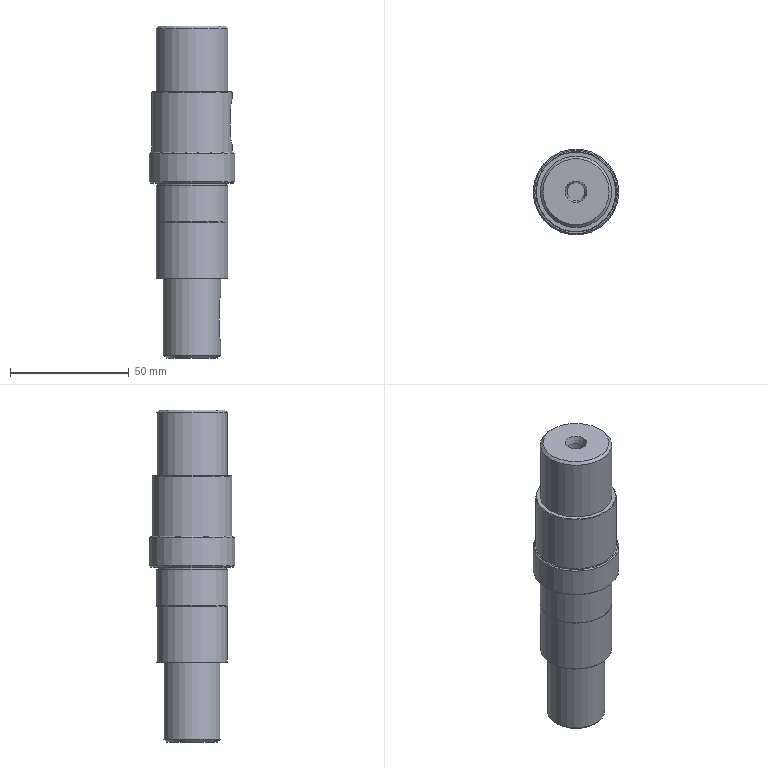Part | NX | features CHAMFER 9, CYLINDER 6, DATUM_CSYS 3, DATUM_PLANE 2, EXTRUDE 2, SKETCH 2, U_SLOT 2, RECT_GROOVE 1, Resize Face 1 | 6 solids | 51 faces | box 36 x 36 x 139.56 mm | volume 97541 mm3 | plane 21 | cylinder 17 | cone 9 | torus 4 | commonest cylinder face diameters 0.8 x2 1 x2 8 x2 10 x2 30 x2 7.48 x1
STEP:
#1=CARTESIAN_POINT('',(-12.04,0.,-110.72));
#2=VERTEX_POINT('',#1);
#3=CARTESIAN_POINT('',(0.,0.,-110.72));
#4=DIRECTION('',(0.,0.,-1.));
#5=DIRECTION('',(-1.,0.,0.));
#6=AXIS2_PLACEMENT_3D('',#3,#4,#5);
#7=CIRCLE('',#6,12.04);
#8=EDGE_CURVE('',#2,#2,#7,.F.);
#9=ORIENTED_EDGE('',*,*,#8,.T.);
#10=EDGE_LOOP('',(#9));
#11=FACE_BOUND('',#10,.T.);
#12=CARTESIAN_POINT('',(11.356,-4.,-89.51));
#13=VERTEX_POINT('',#12);
#14=CARTESIAN_POINT('',(11.356,-4.,-101.11));
#15=VERTEX_POINT('',#14);
#16=CARTESIAN_POINT('',(11.356,-4.,-78.7));
#17=DIRECTION('',(0.,0.,-1.));
#18=VECTOR('',#17,1000.);
#19=LINE('',#16,#18);
#20=EDGE_CURVE('',#13,#15,#19,.T.);
#21=ORIENTED_EDGE('',*,*,#20,.F.);
#22=CARTESIAN_POINT('',(11.356,4.,-89.51));
#23=VERTEX_POINT('',#22);
#24=CARTESIAN_POINT('',(11.356,4.,-89.51));
#25=CARTESIAN_POINT('',(11.356,4.,-88.445));
#26=CARTESIAN_POINT('',(11.708,3.133,-86.386));
#27=CARTESIAN_POINT('',(12.206,0.006902,-85.072));
#28=CARTESIAN_POINT('',(11.708,-3.135,-86.384));
#29=CARTESIAN_POINT('',(11.356,-4.,-88.445));
#30=CARTESIAN_POINT('',(11.356,-4.,-89.51));
#31=B_SPLINE_CURVE_WITH_KNOTS('',3,(#24,#25,#26,#27,#28,#29,#30),.UNSPECIFIED.,.F.,.F.,(4,1,1,1,4),(0.,0.003148,0.006295,0.009443,0.01259),.UNSPECIFIED.);
#32=EDGE_CURVE('',#23,#13,#31,.T.);
#33=ORIENTED_EDGE('',*,*,#32,.F.);
#34=CARTESIAN_POINT('',(11.356,4.,-101.11));
#35=VERTEX_POINT('',#34);
#36=CARTESIAN_POINT('',(11.356,4.,-78.7));
#37=DIRECTION('',(0.,0.,-1.));
#38=VECTOR('',#37,1000.);
#39=LINE('',#36,#38);
#40=EDGE_CURVE('',#35,#23,#39,.F.);
#41=ORIENTED_EDGE('',*,*,#40,.F.);
#42=CARTESIAN_POINT('',(11.356,-4.,-101.11));
#43=CARTESIAN_POINT('',(11.356,-4.,-102.175));
#44=CARTESIAN_POINT('',(11.708,-3.133,-104.234));
#45=CARTESIAN_POINT('',(12.206,-0.006902,-105.548));
#46=CARTESIAN_POINT('',(11.708,3.135,-104.236));
#47=CARTESIAN_POINT('',(11.356,4.,-102.175));
#48=CARTESIAN_POINT('',(11.356,4.,-101.11));
#49=B_SPLINE_CURVE_WITH_KNOTS('',3,(#42,#43,#44,#45,#46,#47,#48),.UNSPECIFIED.,.F.,.F.,(4,1,1,1,4),(0.,0.003148,0.006295,0.009443,0.01259),.UNSPECIFIED.);
#50=EDGE_CURVE('',#15,#35,#49,.T.);
#51=ORIENTED_EDGE('',*,*,#50,.F.);
#52=EDGE_LOOP('',(#21,#33,#41,#51));
#53=FACE_BOUND('',#52,.T.);
#54=CARTESIAN_POINT('',(12.04,0.,-78.7));
#55=VERTEX_POINT('',#54);
#56=CARTESIAN_POINT('',(0.,0.,-78.7));
#57=DIRECTION('',(0.,0.,-1.));
#58=DIRECTION('',(1.,0.,0.));
#59=AXIS2_PLACEMENT_3D('',#56,#57,#58);
#60=CIRCLE('',#59,12.04);
#61=EDGE_CURVE('',#55,#55,#60,.T.);
#62=ORIENTED_EDGE('',*,*,#61,.T.);
#63=EDGE_LOOP('',(#62));
#64=FACE_BOUND('',#63,.T.);
#65=CARTESIAN_POINT('',(0.,0.,-78.7));
#66=DIRECTION('',(0.,0.,-1.));
#67=DIRECTION('',(1.,0.,0.));
#68=AXIS2_PLACEMENT_3D('',#65,#66,#67);
#69=CYLINDRICAL_SURFACE('',#68,12.04);
#70=ADVANCED_FACE('',(#11,#53,#64),#69,.T.);
#71=CARTESIAN_POINT('',(-10.84,0.,-111.92));
#72=VERTEX_POINT('',#71);
#73=CARTESIAN_POINT('',(0.,0.,-111.92));
#74=DIRECTION('',(0.,0.,-1.));
#75=DIRECTION('',(-1.,0.,0.));
#76=AXIS2_PLACEMENT_3D('',#73,#74,#75);
#77=CIRCLE('',#76,10.84);
#78=EDGE_CURVE('',#72,#72,#77,.T.);
#79=ORIENTED_EDGE('',*,*,#78,.T.);
#80=EDGE_LOOP('',(#79));
#81=FACE_BOUND('',#80,.T.);
#82=CARTESIAN_POINT('',(-4.84,0.,-111.92));
#83=VERTEX_POINT('',#82);
#84=CARTESIAN_POINT('',(0.,0.,-111.92));
#85=DIRECTION('',(0.,0.,-1.));
#86=DIRECTION('',(-1.,0.,0.));
#87=AXIS2_PLACEMENT_3D('',#84,#85,#86);
#88=CIRCLE('',#87,4.84);
#89=EDGE_CURVE('',#83,#83,#88,.F.);
#90=ORIENTED_EDGE('',*,*,#89,.T.);
#91=EDGE_LOOP('',(#90));
#92=FACE_BOUND('',#91,.T.);
#93=CARTESIAN_POINT('',(0.,0.,-111.92));
#94=DIRECTION('',(0.,0.,-1.));
#95=DIRECTION('',(-1.,0.,0.));
#96=AXIS2_PLACEMENT_3D('',#93,#94,#95);
#97=PLANE('',#96);
#98=ADVANCED_FACE('',(#81,#92),#97,.T.);
#99=ORIENTED_EDGE('',*,*,#61,.F.);
#100=EDGE_LOOP('',(#99));
#101=FACE_BOUND('',#100,.T.);
#102=CARTESIAN_POINT('',(0.,0.,-78.7));
#103=DIRECTION('',(0.,0.,1.));
#104=DIRECTION('',(1.,0.,0.));
#105=AXIS2_PLACEMENT_3D('',#102,#103,#104);
#106=PLANE('',#105);
#107=ADVANCED_FACE('',(#101),#106,.T.);
#108=CARTESIAN_POINT('',(-4.04,0.,-108.72));
#109=VERTEX_POINT('',#108);
#110=CARTESIAN_POINT('',(0.,0.,-108.72));
#111=DIRECTION('',(0.,0.,-1.));
#112=DIRECTION('',(-1.,0.,0.));
#113=AXIS2_PLACEMENT_3D('',#110,#111,#112);
#114=CIRCLE('',#113,4.04);
#115=EDGE_CURVE('',#109,#109,#114,.T.);
#116=ORIENTED_EDGE('',*,*,#115,.T.);
#117=EDGE_LOOP('',(#116));
#118=FACE_BOUND('',#117,.T.);
#119=CARTESIAN_POINT('',(4.04,0.,-107.02));
#120=VERTEX_POINT('',#119);
#121=CARTESIAN_POINT('',(0.,0.,-107.02));
#122=DIRECTION('',(0.,0.,-1.));
#123=DIRECTION('',(1.,0.,0.));
#124=AXIS2_PLACEMENT_3D('',#121,#122,#123);
#125=CIRCLE('',#124,4.04);
#126=EDGE_CURVE('',#120,#120,#125,.F.);
#127=ORIENTED_EDGE('',*,*,#126,.T.);
#128=EDGE_LOOP('',(#127));
#129=FACE_BOUND('',#128,.T.);
#130=CARTESIAN_POINT('',(0.,0.,-107.02));
#131=DIRECTION('',(0.,0.,-1.));
#132=DIRECTION('',(-1.,0.,0.));
#133=AXIS2_PLACEMENT_3D('',#130,#131,#132);
#134=CYLINDRICAL_SURFACE('',#133,4.04);
#135=ADVANCED_FACE('',(#118,#129),#134,.F.);
#136=ORIENTED_EDGE('',*,*,#126,.F.);
#137=EDGE_LOOP('',(#136));
#138=FACE_BOUND('',#137,.T.);
#139=CARTESIAN_POINT('',(0.,0.,-107.02));
#140=DIRECTION('',(0.,0.,-1.));
#141=DIRECTION('',(-1.,0.,0.));
#142=AXIS2_PLACEMENT_3D('',#139,#140,#141);
#143=PLANE('',#142);
#144=ADVANCED_FACE('',(#138),#143,.T.);
#145=ORIENTED_EDGE('',*,*,#89,.F.);
#146=EDGE_LOOP('',(#145));
#147=FACE_BOUND('',#146,.T.);
#148=ORIENTED_EDGE('',*,*,#115,.F.);
#149=EDGE_LOOP('',(#148));
#150=FACE_BOUND('',#149,.T.);
#151=CARTESIAN_POINT('',(0.,0.,-108.72));
#152=DIRECTION('',(0.,0.,-1.));
#153=DIRECTION('',(-1.,0.,0.));
#154=AXIS2_PLACEMENT_3D('',#151,#152,#153);
#155=CONICAL_SURFACE('',#154,4.04,0.245);
#156=ADVANCED_FACE('',(#147,#150),#155,.F.);
#157=ORIENTED_EDGE('',*,*,#20,.T.);
#158=CARTESIAN_POINT('',(9.34,-4.,-101.11));
#159=VERTEX_POINT('',#158);
#160=CARTESIAN_POINT('',(12.04,-4.,-101.11));
#161=DIRECTION('',(1.,0.,0.));
#162=VECTOR('',#161,1000.);
#163=LINE('',#160,#162);
#164=EDGE_CURVE('',#15,#159,#163,.F.);
#165=ORIENTED_EDGE('',*,*,#164,.T.);
#166=CARTESIAN_POINT('',(9.34,-4.,-89.51));
#167=VERTEX_POINT('',#166);
#168=CARTESIAN_POINT('',(9.34,-4.,-101.11));
#169=DIRECTION('',(0.,0.,1.));
#170=VECTOR('',#169,1000.);
#171=LINE('',#168,#170);
#172=EDGE_CURVE('',#167,#159,#171,.F.);
#173=ORIENTED_EDGE('',*,*,#172,.F.);
#174=CARTESIAN_POINT('',(12.04,-4.,-89.51));
#175=DIRECTION('',(1.,0.,0.));
#176=VECTOR('',#175,1000.);
#177=LINE('',#174,#176);
#178=EDGE_CURVE('',#13,#167,#177,.F.);
#179=ORIENTED_EDGE('',*,*,#178,.F.);
#180=EDGE_LOOP('',(#157,#165,#173,#179));
#181=FACE_BOUND('',#180,.T.);
#182=CARTESIAN_POINT('',(12.04,-4.,-95.31));
#183=DIRECTION('',(0.,-1.,0.));
#184=DIRECTION('',(0.,0.,-1.));
#185=AXIS2_PLACEMENT_3D('',#182,#183,#184);
#186=PLANE('',#185);
#187=ADVANCED_FACE('',(#181),#186,.F.);
#188=ORIENTED_EDGE('',*,*,#172,.T.);
#189=CARTESIAN_POINT('',(8.94,-3.6,-101.11));
#190=VERTEX_POINT('',#189);
#191=CARTESIAN_POINT('',(9.34,-3.6,-101.11));
#192=DIRECTION('',(0.,0.,1.));
#193=DIRECTION('',(1.,0.,0.));
#194=AXIS2_PLACEMENT_3D('',#191,#192,#193);
#195=CIRCLE('',#194,0.4);
#196=EDGE_CURVE('',#159,#190,#195,.F.);
#197=ORIENTED_EDGE('',*,*,#196,.T.);
#198=CARTESIAN_POINT('',(8.94,-3.6,-89.51));
#199=VERTEX_POINT('',#198);
#200=CARTESIAN_POINT('',(8.94,-3.6,-95.31));
#201=DIRECTION('',(0.,0.,1.));
#202=VECTOR('',#201,1000.);
#203=LINE('',#200,#202);
#204=EDGE_CURVE('',#199,#190,#203,.F.);
#205=ORIENTED_EDGE('',*,*,#204,.F.);
#206=CARTESIAN_POINT('',(9.34,-3.6,-89.51));
#207=DIRECTION('',(0.,0.,1.));
#208=DIRECTION('',(1.,0.,0.));
#209=AXIS2_PLACEMENT_3D('',#206,#207,#208);
#210=CIRCLE('',#209,0.4);
#211=EDGE_CURVE('',#167,#199,#210,.F.);
#212=ORIENTED_EDGE('',*,*,#211,.F.);
#213=EDGE_LOOP('',(#188,#197,#205,#212));
#214=FACE_BOUND('',#213,.T.);
#215=CARTESIAN_POINT('',(9.34,-3.6,-95.31));
#216=DIRECTION('',(0.,0.,1.));
#217=DIRECTION('',(1.,0.,0.));
#218=AXIS2_PLACEMENT_3D('',#215,#216,#217);
#219=CYLINDRICAL_SURFACE('',#218,0.4);
#220=ADVANCED_FACE('',(#214),#219,.F.);
#221=ORIENTED_EDGE('',*,*,#204,.T.);
#222=CARTESIAN_POINT('',(8.94,3.6,-101.11));
#223=VERTEX_POINT('',#222);
#224=CARTESIAN_POINT('',(8.94,0.,-101.11));
#225=DIRECTION('',(1.,0.,0.));
#226=DIRECTION('',(0.,0.,-1.));
#227=AXIS2_PLACEMENT_3D('',#224,#225,#226);
#228=CIRCLE('',#227,3.6);
#229=EDGE_CURVE('',#223,#190,#228,.F.);
#230=ORIENTED_EDGE('',*,*,#229,.F.);
#231=CARTESIAN_POINT('',(8.94,3.6,-89.51));
#232=VERTEX_POINT('',#231);
#233=CARTESIAN_POINT('',(8.94,3.6,-95.31));
#234=DIRECTION('',(0.,0.,1.));
#235=VECTOR('',#234,1000.);
#236=LINE('',#233,#235);
#237=EDGE_CURVE('',#232,#223,#236,.F.);
#238=ORIENTED_EDGE('',*,*,#237,.F.);
#239=CARTESIAN_POINT('',(8.94,0.,-89.51));
#240=DIRECTION('',(1.,0.,0.));
#241=DIRECTION('',(0.,0.,-1.));
#242=AXIS2_PLACEMENT_3D('',#239,#240,#241);
#243=CIRCLE('',#242,3.6);
#244=EDGE_CURVE('',#199,#232,#243,.F.);
#245=ORIENTED_EDGE('',*,*,#244,.F.);
#246=EDGE_LOOP('',(#221,#230,#238,#245));
#247=FACE_BOUND('',#246,.T.);
#248=CARTESIAN_POINT('',(8.94,0.,-95.31));
#249=DIRECTION('',(-1.,0.,0.));
#250=DIRECTION('',(0.,0.,1.));
#251=AXIS2_PLACEMENT_3D('',#248,#249,#250);
#252=PLANE('',#251);
#253=ADVANCED_FACE('',(#247),#252,.F.);
#254=ORIENTED_EDGE('',*,*,#237,.T.);
#255=CARTESIAN_POINT('',(9.34,4.,-101.11));
#256=VERTEX_POINT('',#255);
#257=CARTESIAN_POINT('',(9.34,3.6,-101.11));
#258=DIRECTION('',(0.,0.,1.));
#259=DIRECTION('',(1.,0.,0.));
#260=AXIS2_PLACEMENT_3D('',#257,#258,#259);
#261=CIRCLE('',#260,0.4);
#262=EDGE_CURVE('',#223,#256,#261,.F.);
#263=ORIENTED_EDGE('',*,*,#262,.T.);
#264=CARTESIAN_POINT('',(9.34,4.,-89.51));
#265=VERTEX_POINT('',#264);
#266=CARTESIAN_POINT('',(9.34,4.,-101.11));
#267=DIRECTION('',(0.,0.,1.));
#268=VECTOR('',#267,1000.);
#269=LINE('',#266,#268);
#270=EDGE_CURVE('',#265,#256,#269,.F.);
#271=ORIENTED_EDGE('',*,*,#270,.F.);
#272=CARTESIAN_POINT('',(9.34,3.6,-89.51));
#273=DIRECTION('',(0.,0.,1.));
#274=DIRECTION('',(1.,0.,0.));
#275=AXIS2_PLACEMENT_3D('',#272,#273,#274);
#276=CIRCLE('',#275,0.4);
#277=EDGE_CURVE('',#232,#265,#276,.F.);
#278=ORIENTED_EDGE('',*,*,#277,.F.);
#279=EDGE_LOOP('',(#254,#263,#271,#278));
#280=FACE_BOUND('',#279,.T.);
#281=CARTESIAN_POINT('',(9.34,3.6,-95.31));
#282=DIRECTION('',(0.,0.,1.));
#283=DIRECTION('',(1.,0.,0.));
#284=AXIS2_PLACEMENT_3D('',#281,#282,#283);
#285=CYLINDRICAL_SURFACE('',#284,0.4);
#286=ADVANCED_FACE('',(#280),#285,.F.);
#287=ORIENTED_EDGE('',*,*,#32,.T.);
#288=ORIENTED_EDGE('',*,*,#178,.T.);
#289=CARTESIAN_POINT('',(9.34,0.,-89.51));
#290=DIRECTION('',(1.,0.,0.));
#291=DIRECTION('',(0.,0.,-1.));
#292=AXIS2_PLACEMENT_3D('',#289,#290,#291);
#293=CIRCLE('',#292,4.);
#294=EDGE_CURVE('',#167,#265,#293,.F.);
#295=ORIENTED_EDGE('',*,*,#294,.T.);
#296=CARTESIAN_POINT('',(12.04,4.,-89.51));
#297=DIRECTION('',(1.,0.,0.));
#298=VECTOR('',#297,1000.);
#299=LINE('',#296,#298);
#300=EDGE_CURVE('',#23,#265,#299,.F.);
#301=ORIENTED_EDGE('',*,*,#300,.F.);
#302=EDGE_LOOP('',(#287,#288,#295,#301));
#303=FACE_BOUND('',#302,.T.);
#304=CARTESIAN_POINT('',(12.04,0.,-89.51));
#305=DIRECTION('',(1.,0.,0.));
#306=DIRECTION('',(0.,0.,-1.));
#307=AXIS2_PLACEMENT_3D('',#304,#305,#306);
#308=CYLINDRICAL_SURFACE('',#307,4.);
#309=ADVANCED_FACE('',(#303),#308,.F.);
#310=ORIENTED_EDGE('',*,*,#40,.T.);
#311=ORIENTED_EDGE('',*,*,#300,.T.);
#312=ORIENTED_EDGE('',*,*,#270,.T.);
#313=CARTESIAN_POINT('',(12.04,4.,-101.11));
#314=DIRECTION('',(1.,0.,0.));
#315=VECTOR('',#314,1000.);
#316=LINE('',#313,#315);
#317=EDGE_CURVE('',#35,#256,#316,.F.);
#318=ORIENTED_EDGE('',*,*,#317,.F.);
#319=EDGE_LOOP('',(#310,#311,#312,#318));
#320=FACE_BOUND('',#319,.T.);
#321=CARTESIAN_POINT('',(12.04,4.,-95.31));
#322=DIRECTION('',(0.,1.,0.));
#323=DIRECTION('',(0.,0.,1.));
#324=AXIS2_PLACEMENT_3D('',#321,#322,#323);
#325=PLANE('',#324);
#326=ADVANCED_FACE('',(#320),#325,.F.);
#327=ORIENTED_EDGE('',*,*,#164,.F.);
#328=ORIENTED_EDGE('',*,*,#50,.T.);
#329=ORIENTED_EDGE('',*,*,#317,.T.);
#330=CARTESIAN_POINT('',(9.34,0.,-101.11));
#331=DIRECTION('',(1.,0.,0.));
#332=DIRECTION('',(0.,0.,-1.));
#333=AXIS2_PLACEMENT_3D('',#330,#331,#332);
#334=CIRCLE('',#333,4.);
#335=EDGE_CURVE('',#256,#159,#334,.F.);
#336=ORIENTED_EDGE('',*,*,#335,.T.);
#337=EDGE_LOOP('',(#327,#328,#329,#336));
#338=FACE_BOUND('',#337,.T.);
#339=CARTESIAN_POINT('',(12.04,0.,-101.11));
#340=DIRECTION('',(1.,0.,0.));
#341=DIRECTION('',(0.,0.,-1.));
#342=AXIS2_PLACEMENT_3D('',#339,#340,#341);
#343=CYLINDRICAL_SURFACE('',#342,4.);
#344=ADVANCED_FACE('',(#338),#343,.F.);
#345=ORIENTED_EDGE('',*,*,#244,.T.);
#346=ORIENTED_EDGE('',*,*,#277,.T.);
#347=ORIENTED_EDGE('',*,*,#294,.F.);
#348=ORIENTED_EDGE('',*,*,#211,.T.);
#349=EDGE_LOOP('',(#345,#346,#347,#348));
#350=FACE_BOUND('',#349,.T.);
#351=CARTESIAN_POINT('',(9.34,0.,-89.51));
#352=DIRECTION('',(1.,0.,0.));
#353=DIRECTION('',(0.,0.,-1.));
#354=AXIS2_PLACEMENT_3D('',#351,#352,#353);
#355=TOROIDAL_SURFACE('',#354,3.6,0.4);
#356=ADVANCED_FACE('',(#350),#355,.F.);
#357=ORIENTED_EDGE('',*,*,#229,.T.);
#358=ORIENTED_EDGE('',*,*,#196,.F.);
#359=ORIENTED_EDGE('',*,*,#335,.F.);
#360=ORIENTED_EDGE('',*,*,#262,.F.);
#361=EDGE_LOOP('',(#357,#358,#359,#360));
#362=FACE_BOUND('',#361,.T.);
#363=CARTESIAN_POINT('',(9.34,0.,-101.11));
#364=DIRECTION('',(1.,0.,0.));
#365=DIRECTION('',(0.,0.,-1.));
#366=AXIS2_PLACEMENT_3D('',#363,#364,#365);
#367=TOROIDAL_SURFACE('',#366,3.6,0.4);
#368=ADVANCED_FACE('',(#362),#367,.F.);
#369=ORIENTED_EDGE('',*,*,#78,.F.);
#370=EDGE_LOOP('',(#369));
#371=FACE_BOUND('',#370,.T.);
#372=ORIENTED_EDGE('',*,*,#8,.F.);
#373=EDGE_LOOP('',(#372));
#374=FACE_BOUND('',#373,.T.);
#375=CARTESIAN_POINT('',(0.,0.,-110.72));
#376=DIRECTION('',(0.,0.,1.));
#377=DIRECTION('',(1.,0.,0.));
#378=AXIS2_PLACEMENT_3D('',#375,#376,#377);
#379=CONICAL_SURFACE('',#378,12.04,0.7854);
#380=ADVANCED_FACE('',(#371,#374),#379,.T.);
#381=CLOSED_SHELL('',(#70,#98,#107,#135,#144,#156,#187,#220,#253,#286,#309,#326,#344,#356,#368,#380));
#382=MANIFOLD_SOLID_BREP('',#381);
#383=CARTESIAN_POINT('',(-14.6,0.,-78.7));
#384=VERTEX_POINT('',#383);
#385=CARTESIAN_POINT('',(0.,0.,-78.7));
#386=DIRECTION('',(0.,0.,-1.));
#387=DIRECTION('',(-1.,0.,0.));
#388=AXIS2_PLACEMENT_3D('',#385,#386,#387);
#389=CIRCLE('',#388,14.6);
#390=EDGE_CURVE('',#384,#384,#389,.T.);
#391=ORIENTED_EDGE('',*,*,#390,.T.);
#392=EDGE_LOOP('',(#391));
#393=FACE_BOUND('',#392,.T.);
#394=CARTESIAN_POINT('',(0.,0.,-78.7));
#395=DIRECTION('',(0.,0.,-1.));
#396=DIRECTION('',(-1.,0.,0.));
#397=AXIS2_PLACEMENT_3D('',#394,#395,#396);
#398=PLANE('',#397);
#399=ADVANCED_FACE('',(#393),#398,.T.);
#400=CARTESIAN_POINT('',(15.,0.,-54.76));
#401=VERTEX_POINT('',#400);
#402=CARTESIAN_POINT('',(0.,0.,-54.76));
#403=DIRECTION('',(0.,0.,1.));
#404=DIRECTION('',(1.,0.,0.));
#405=AXIS2_PLACEMENT_3D('',#402,#403,#404);
#406=CIRCLE('',#405,15.);
#407=EDGE_CURVE('',#401,#401,#406,.F.);
#408=ORIENTED_EDGE('',*,*,#407,.F.);
#409=EDGE_LOOP('',(#408));
#410=FACE_BOUND('',#409,.T.);
#411=CARTESIAN_POINT('',(0.,0.,-54.76));
#412=DIRECTION('',(0.,0.,1.));
#413=DIRECTION('',(1.,0.,0.));
#414=AXIS2_PLACEMENT_3D('',#411,#412,#413);
#415=PLANE('',#414);
#416=ADVANCED_FACE('',(#410),#415,.T.);
#417=CARTESIAN_POINT('',(15.,0.,-78.3));
#418=VERTEX_POINT('',#417);
#419=CARTESIAN_POINT('',(0.,0.,-78.3));
#420=DIRECTION('',(0.,0.,1.));
#421=DIRECTION('',(1.,0.,0.));
#422=AXIS2_PLACEMENT_3D('',#419,#420,#421);
#423=CIRCLE('',#422,15.);
#424=EDGE_CURVE('',#418,#418,#423,.T.);
#425=ORIENTED_EDGE('',*,*,#424,.T.);
#426=EDGE_LOOP('',(#425));
#427=FACE_BOUND('',#426,.T.);
#428=ORIENTED_EDGE('',*,*,#407,.T.);
#429=EDGE_LOOP('',(#428));
#430=FACE_BOUND('',#429,.T.);
#431=CARTESIAN_POINT('',(0.,0.,-54.76));
#432=DIRECTION('',(0.,0.,-1.));
#433=DIRECTION('',(1.,0.,0.));
#434=AXIS2_PLACEMENT_3D('',#431,#432,#433);
#435=CYLINDRICAL_SURFACE('',#434,15.);
#436=ADVANCED_FACE('',(#427,#430),#435,.T.);
#437=ORIENTED_EDGE('',*,*,#390,.F.);
#438=EDGE_LOOP('',(#437));
#439=FACE_BOUND('',#438,.T.);
#440=ORIENTED_EDGE('',*,*,#424,.F.);
#441=EDGE_LOOP('',(#440));
#442=FACE_BOUND('',#441,.T.);
#443=CARTESIAN_POINT('',(0.,0.,-78.3));
#444=DIRECTION('',(0.,0.,1.));
#445=DIRECTION('',(1.,0.,0.));
#446=AXIS2_PLACEMENT_3D('',#443,#444,#445);
#447=CONICAL_SURFACE('',#446,15.,0.7854);
#448=ADVANCED_FACE('',(#439,#442),#447,.T.);
#449=CLOSED_SHELL('',(#399,#416,#436,#448));
#450=MANIFOLD_SOLID_BREP('',#449);
#451=CARTESIAN_POINT('',(13.9,0.,27.64));
#452=VERTEX_POINT('',#451);
#453=CARTESIAN_POINT('',(0.,0.,27.64));
#454=DIRECTION('',(0.,0.,1.));
#455=DIRECTION('',(1.,0.,0.));
#456=AXIS2_PLACEMENT_3D('',#453,#454,#455);
#457=CIRCLE('',#456,13.9);
#458=EDGE_CURVE('',#452,#452,#457,.T.);
#459=ORIENTED_EDGE('',*,*,#458,.T.);
#460=EDGE_LOOP('',(#459));
#461=FACE_BOUND('',#460,.T.);
#462=CARTESIAN_POINT('',(4.54,0.,27.64));
#463=VERTEX_POINT('',#462);
#464=CARTESIAN_POINT('',(0.,0.,27.64));
#465=DIRECTION('',(0.,0.,1.));
#466=DIRECTION('',(1.,0.,0.));
#467=AXIS2_PLACEMENT_3D('',#464,#465,#466);
#468=CIRCLE('',#467,4.54);
#469=EDGE_CURVE('',#463,#463,#468,.F.);
#470=ORIENTED_EDGE('',*,*,#469,.T.);
#471=EDGE_LOOP('',(#470));
#472=FACE_BOUND('',#471,.T.);
#473=CARTESIAN_POINT('',(0.,0.,27.64));
#474=DIRECTION('',(0.,0.,1.));
#475=DIRECTION('',(1.,0.,0.));
#476=AXIS2_PLACEMENT_3D('',#473,#474,#475);
#477=PLANE('',#476);
#478=ADVANCED_FACE('',(#461,#472),#477,.T.);
#479=CARTESIAN_POINT('',(15.,0.,0.));
#480=VERTEX_POINT('',#479);
#481=CARTESIAN_POINT('',(0.,0.,0.));
#482=DIRECTION('',(0.,0.,1.));
#483=DIRECTION('',(1.,0.,0.));
#484=AXIS2_PLACEMENT_3D('',#481,#482,#483);
#485=CIRCLE('',#484,15.);
#486=EDGE_CURVE('',#480,#480,#485,.T.);
#487=ORIENTED_EDGE('',*,*,#486,.F.);
#488=EDGE_LOOP('',(#487));
#489=FACE_BOUND('',#488,.T.);
#490=CARTESIAN_POINT('',(0.,0.,0.));
#491=DIRECTION('',(0.,0.,-1.));
#492=DIRECTION('',(-1.,0.,0.));
#493=AXIS2_PLACEMENT_3D('',#490,#491,#492);
#494=PLANE('',#493);
#495=ADVANCED_FACE('',(#489),#494,.T.);
#496=CARTESIAN_POINT('',(15.,0.,26.54));
#497=VERTEX_POINT('',#496);
#498=CARTESIAN_POINT('',(0.,0.,26.54));
#499=DIRECTION('',(0.,0.,1.));
#500=DIRECTION('',(1.,0.,0.));
#501=AXIS2_PLACEMENT_3D('',#498,#499,#500);
#502=CIRCLE('',#501,15.);
#503=EDGE_CURVE('',#497,#497,#502,.F.);
#504=ORIENTED_EDGE('',*,*,#503,.T.);
#505=EDGE_LOOP('',(#504));
#506=FACE_BOUND('',#505,.T.);
#507=ORIENTED_EDGE('',*,*,#486,.T.);
#508=EDGE_LOOP('',(#507));
#509=FACE_BOUND('',#508,.T.);
#510=CARTESIAN_POINT('',(0.,0.,0.));
#511=DIRECTION('',(0.,0.,1.));
#512=DIRECTION('',(1.,0.,0.));
#513=AXIS2_PLACEMENT_3D('',#510,#511,#512);
#514=CYLINDRICAL_SURFACE('',#513,15.);
#515=ADVANCED_FACE('',(#506,#509),#514,.T.);
#516=CARTESIAN_POINT('',(3.74,0.,24.44));
#517=VERTEX_POINT('',#516);
#518=CARTESIAN_POINT('',(0.,0.,24.44));
#519=DIRECTION('',(0.,0.,1.));
#520=DIRECTION('',(1.,0.,0.));
#521=AXIS2_PLACEMENT_3D('',#518,#519,#520);
#522=CIRCLE('',#521,3.74);
#523=EDGE_CURVE('',#517,#517,#522,.T.);
#524=ORIENTED_EDGE('',*,*,#523,.T.);
#525=EDGE_LOOP('',(#524));
#526=FACE_BOUND('',#525,.T.);
#527=CARTESIAN_POINT('',(3.74,0.,21.24));
#528=VERTEX_POINT('',#527);
#529=CARTESIAN_POINT('',(0.,0.,21.24));
#530=DIRECTION('',(0.,0.,1.));
#531=DIRECTION('',(1.,0.,0.));
#532=AXIS2_PLACEMENT_3D('',#529,#530,#531);
#533=CIRCLE('',#532,3.74);
#534=EDGE_CURVE('',#528,#528,#533,.F.);
#535=ORIENTED_EDGE('',*,*,#534,.T.);
#536=EDGE_LOOP('',(#535));
#537=FACE_BOUND('',#536,.T.);
#538=CARTESIAN_POINT('',(0.,0.,21.24));
#539=DIRECTION('',(0.,0.,1.));
#540=DIRECTION('',(1.,0.,0.));
#541=AXIS2_PLACEMENT_3D('',#538,#539,#540);
#542=CYLINDRICAL_SURFACE('',#541,3.74);
#543=ADVANCED_FACE('',(#526,#537),#542,.F.);
#544=ORIENTED_EDGE('',*,*,#534,.F.);
#545=EDGE_LOOP('',(#544));
#546=FACE_BOUND('',#545,.T.);
#547=CARTESIAN_POINT('',(0.,0.,21.24));
#548=DIRECTION('',(0.,0.,1.));
#549=DIRECTION('',(1.,0.,0.));
#550=AXIS2_PLACEMENT_3D('',#547,#548,#549);
#551=PLANE('',#550);
#552=ADVANCED_FACE('',(#546),#551,.T.);
#553=ORIENTED_EDGE('',*,*,#469,.F.);
#554=EDGE_LOOP('',(#553));
#555=FACE_BOUND('',#554,.T.);
#556=ORIENTED_EDGE('',*,*,#523,.F.);
#557=EDGE_LOOP('',(#556));
#558=FACE_BOUND('',#557,.T.);
#559=CARTESIAN_POINT('',(0.,0.,24.44));
#560=DIRECTION('',(0.,0.,1.));
#561=DIRECTION('',(1.,0.,0.));
#562=AXIS2_PLACEMENT_3D('',#559,#560,#561);
#563=CONICAL_SURFACE('',#562,3.74,0.245);
#564=ADVANCED_FACE('',(#555,#558),#563,.F.);
#565=ORIENTED_EDGE('',*,*,#458,.F.);
#566=EDGE_LOOP('',(#565));
#567=FACE_BOUND('',#566,.T.);
#568=ORIENTED_EDGE('',*,*,#503,.F.);
#569=EDGE_LOOP('',(#568));
#570=FACE_BOUND('',#569,.T.);
#571=CARTESIAN_POINT('',(0.,0.,26.54));
#572=DIRECTION('',(0.,0.,-1.));
#573=DIRECTION('',(-1.,0.,0.));
#574=AXIS2_PLACEMENT_3D('',#571,#572,#573);
#575=CONICAL_SURFACE('',#574,15.,0.7854);
#576=ADVANCED_FACE('',(#567,#570),#575,.T.);
#577=CLOSED_SHELL('',(#478,#495,#515,#543,#552,#564,#576));
#578=MANIFOLD_SOLID_BREP('',#577);
#579=CARTESIAN_POINT('',(16.9,0.,-0.2));
#580=VERTEX_POINT('',#579);
#581=CARTESIAN_POINT('',(0.,0.,-0.2));
#582=DIRECTION('',(0.,0.,1.));
#583=DIRECTION('',(1.,0.,0.));
#584=AXIS2_PLACEMENT_3D('',#581,#582,#583);
#585=CIRCLE('',#584,16.9);
#586=EDGE_CURVE('',#580,#580,#585,.F.);
#587=ORIENTED_EDGE('',*,*,#586,.T.);
#588=EDGE_LOOP('',(#587));
#589=FACE_BOUND('',#588,.T.);
#590=CARTESIAN_POINT('',(16.143,-5.,-7.88));
#591=VERTEX_POINT('',#590);
#592=CARTESIAN_POINT('',(16.143,-5.,-17.48));
#593=VERTEX_POINT('',#592);
#594=CARTESIAN_POINT('',(16.143,-5.,0.));
#595=DIRECTION('',(0.,0.,-1.));
#596=VECTOR('',#595,1000.);
#597=LINE('',#594,#596);
#598=EDGE_CURVE('',#591,#593,#597,.T.);
#599=ORIENTED_EDGE('',*,*,#598,.F.);
#600=CARTESIAN_POINT('',(16.143,5.,-7.88));
#601=VERTEX_POINT('',#600);
#602=CARTESIAN_POINT('',(16.143,5.,-7.88));
#603=CARTESIAN_POINT('',(16.143,5.,-6.551));
#604=CARTESIAN_POINT('',(16.53,3.916,-3.974));
#605=CARTESIAN_POINT('',(17.085,0.007874,-2.334));
#606=CARTESIAN_POINT('',(16.531,-3.918,-3.971));
#607=CARTESIAN_POINT('',(16.143,-5.,-6.551));
#608=CARTESIAN_POINT('',(16.143,-5.,-7.88));
#609=B_SPLINE_CURVE_WITH_KNOTS('',3,(#602,#603,#604,#605,#606,#607,#608),.UNSPECIFIED.,.F.,.F.,(4,1,1,1,4),(0.,0.003929,0.007858,0.01179,0.01572),.UNSPECIFIED.);
#610=EDGE_CURVE('',#601,#591,#609,.T.);
#611=ORIENTED_EDGE('',*,*,#610,.F.);
#612=CARTESIAN_POINT('',(16.143,5.,-17.48));
#613=VERTEX_POINT('',#612);
#614=CARTESIAN_POINT('',(16.143,5.,0.));
#615=DIRECTION('',(0.,0.,-1.));
#616=VECTOR('',#615,1000.);
#617=LINE('',#614,#616);
#618=EDGE_CURVE('',#613,#601,#617,.F.);
#619=ORIENTED_EDGE('',*,*,#618,.F.);
#620=CARTESIAN_POINT('',(16.143,-5.,-17.48));
#621=CARTESIAN_POINT('',(16.143,-5.,-18.809));
#622=CARTESIAN_POINT('',(16.53,-3.916,-21.386));
#623=CARTESIAN_POINT('',(17.085,-0.007874,-23.026));
#624=CARTESIAN_POINT('',(16.531,3.918,-21.389));
#625=CARTESIAN_POINT('',(16.143,5.,-18.809));
#626=CARTESIAN_POINT('',(16.143,5.,-17.48));
#627=B_SPLINE_CURVE_WITH_KNOTS('',3,(#620,#621,#622,#623,#624,#625,#626),.UNSPECIFIED.,.F.,.F.,(4,1,1,1,4),(0.,0.003929,0.007858,0.01179,0.01572),.UNSPECIFIED.);
#628=EDGE_CURVE('',#593,#613,#627,.T.);
#629=ORIENTED_EDGE('',*,*,#628,.F.);
#630=EDGE_LOOP('',(#599,#611,#619,#629));
#631=FACE_BOUND('',#630,.T.);
#632=CARTESIAN_POINT('',(16.9,0.,-25.36));
#633=VERTEX_POINT('',#632);
#634=CARTESIAN_POINT('',(0.,0.,-25.36));
#635=DIRECTION('',(0.,0.,1.));
#636=DIRECTION('',(1.,0.,0.));
#637=AXIS2_PLACEMENT_3D('',#634,#635,#636);
#638=CIRCLE('',#637,16.9);
#639=EDGE_CURVE('',#633,#633,#638,.T.);
#640=ORIENTED_EDGE('',*,*,#639,.T.);
#641=EDGE_LOOP('',(#640));
#642=FACE_BOUND('',#641,.T.);
#643=CARTESIAN_POINT('',(0.,0.,0.));
#644=DIRECTION('',(0.,0.,-1.));
#645=DIRECTION('',(1.,0.,0.));
#646=AXIS2_PLACEMENT_3D('',#643,#644,#645);
#647=CYLINDRICAL_SURFACE('',#646,16.9);
#648=ADVANCED_FACE('',(#589,#631,#642),#647,.T.);
#649=ORIENTED_EDGE('',*,*,#639,.F.);
#650=EDGE_LOOP('',(#649));
#651=FACE_BOUND('',#650,.T.);
#652=CARTESIAN_POINT('',(0.,0.,-25.36));
#653=DIRECTION('',(0.,0.,-1.));
#654=DIRECTION('',(-1.,0.,0.));
#655=AXIS2_PLACEMENT_3D('',#652,#653,#654);
#656=PLANE('',#655);
#657=ADVANCED_FACE('',(#651),#656,.T.);
#658=CARTESIAN_POINT('',(16.7,0.,0.));
#659=VERTEX_POINT('',#658);
#660=CARTESIAN_POINT('',(0.,0.,0.));
#661=DIRECTION('',(0.,0.,1.));
#662=DIRECTION('',(1.,0.,0.));
#663=AXIS2_PLACEMENT_3D('',#660,#661,#662);
#664=CIRCLE('',#663,16.7);
#665=EDGE_CURVE('',#659,#659,#664,.T.);
#666=ORIENTED_EDGE('',*,*,#665,.T.);
#667=EDGE_LOOP('',(#666));
#668=FACE_BOUND('',#667,.T.);
#669=CARTESIAN_POINT('',(0.,0.,0.));
#670=DIRECTION('',(0.,0.,1.));
#671=DIRECTION('',(1.,0.,0.));
#672=AXIS2_PLACEMENT_3D('',#669,#670,#671);
#673=PLANE('',#672);
#674=ADVANCED_FACE('',(#668),#673,.T.);
#675=ORIENTED_EDGE('',*,*,#598,.T.);
#676=CARTESIAN_POINT('',(13.94,-5.,-17.48));
#677=VERTEX_POINT('',#676);
#678=CARTESIAN_POINT('',(16.9,-5.,-17.48));
#679=DIRECTION('',(1.,0.,0.));
#680=VECTOR('',#679,1000.);
#681=LINE('',#678,#680);
#682=EDGE_CURVE('',#593,#677,#681,.F.);
#683=ORIENTED_EDGE('',*,*,#682,.T.);
#684=CARTESIAN_POINT('',(13.94,-5.,-7.88));
#685=VERTEX_POINT('',#684);
#686=CARTESIAN_POINT('',(13.94,-5.,-17.48));
#687=DIRECTION('',(0.,0.,1.));
#688=VECTOR('',#687,1000.);
#689=LINE('',#686,#688);
#690=EDGE_CURVE('',#685,#677,#689,.F.);
#691=ORIENTED_EDGE('',*,*,#690,.F.);
#692=CARTESIAN_POINT('',(16.9,-5.,-7.88));
#693=DIRECTION('',(1.,0.,0.));
#694=VECTOR('',#693,1000.);
#695=LINE('',#692,#694);
#696=EDGE_CURVE('',#591,#685,#695,.F.);
#697=ORIENTED_EDGE('',*,*,#696,.F.);
#698=EDGE_LOOP('',(#675,#683,#691,#697));
#699=FACE_BOUND('',#698,.T.);
#700=CARTESIAN_POINT('',(16.9,-5.,-12.68));
#701=DIRECTION('',(0.,-1.,0.));
#702=DIRECTION('',(0.,0.,-1.));
#703=AXIS2_PLACEMENT_3D('',#700,#701,#702);
#704=PLANE('',#703);
#705=ADVANCED_FACE('',(#699),#704,.F.);
#706=ORIENTED_EDGE('',*,*,#690,.T.);
#707=CARTESIAN_POINT('',(13.44,-4.5,-17.48));
#708=VERTEX_POINT('',#707);
#709=CARTESIAN_POINT('',(13.94,-4.5,-17.48));
#710=DIRECTION('',(0.,0.,1.));
#711=DIRECTION('',(1.,0.,0.));
#712=AXIS2_PLACEMENT_3D('',#709,#710,#711);
#713=CIRCLE('',#712,0.5);
#714=EDGE_CURVE('',#677,#708,#713,.F.);
#715=ORIENTED_EDGE('',*,*,#714,.T.);
#716=CARTESIAN_POINT('',(13.44,-4.5,-7.88));
#717=VERTEX_POINT('',#716);
#718=CARTESIAN_POINT('',(13.44,-4.5,-12.68));
#719=DIRECTION('',(0.,0.,1.));
#720=VECTOR('',#719,1000.);
#721=LINE('',#718,#720);
#722=EDGE_CURVE('',#717,#708,#721,.F.);
#723=ORIENTED_EDGE('',*,*,#722,.F.);
#724=CARTESIAN_POINT('',(13.94,-4.5,-7.88));
#725=DIRECTION('',(0.,0.,1.));
#726=DIRECTION('',(1.,0.,0.));
#727=AXIS2_PLACEMENT_3D('',#724,#725,#726);
#728=CIRCLE('',#727,0.5);
#729=EDGE_CURVE('',#685,#717,#728,.F.);
#730=ORIENTED_EDGE('',*,*,#729,.F.);
#731=EDGE_LOOP('',(#706,#715,#723,#730));
#732=FACE_BOUND('',#731,.T.);
#733=CARTESIAN_POINT('',(13.94,-4.5,-12.68));
#734=DIRECTION('',(0.,0.,1.));
#735=DIRECTION('',(1.,0.,0.));
#736=AXIS2_PLACEMENT_3D('',#733,#734,#735);
#737=CYLINDRICAL_SURFACE('',#736,0.5);
#738=ADVANCED_FACE('',(#732),#737,.F.);
#739=ORIENTED_EDGE('',*,*,#722,.T.);
#740=CARTESIAN_POINT('',(13.44,4.5,-17.48));
#741=VERTEX_POINT('',#740);
#742=CARTESIAN_POINT('',(13.44,0.,-17.48));
#743=DIRECTION('',(1.,0.,0.));
#744=DIRECTION('',(0.,0.,-1.));
#745=AXIS2_PLACEMENT_3D('',#742,#743,#744);
#746=CIRCLE('',#745,4.5);
#747=EDGE_CURVE('',#741,#708,#746,.F.);
#748=ORIENTED_EDGE('',*,*,#747,.F.);
#749=CARTESIAN_POINT('',(13.44,4.5,-7.88));
#750=VERTEX_POINT('',#749);
#751=CARTESIAN_POINT('',(13.44,4.5,-12.68));
#752=DIRECTION('',(0.,0.,1.));
#753=VECTOR('',#752,1000.);
#754=LINE('',#751,#753);
#755=EDGE_CURVE('',#750,#741,#754,.F.);
#756=ORIENTED_EDGE('',*,*,#755,.F.);
#757=CARTESIAN_POINT('',(13.44,0.,-7.88));
#758=DIRECTION('',(1.,0.,0.));
#759=DIRECTION('',(0.,0.,-1.));
#760=AXIS2_PLACEMENT_3D('',#757,#758,#759);
#761=CIRCLE('',#760,4.5);
#762=EDGE_CURVE('',#717,#750,#761,.F.);
#763=ORIENTED_EDGE('',*,*,#762,.F.);
#764=EDGE_LOOP('',(#739,#748,#756,#763));
#765=FACE_BOUND('',#764,.T.);
#766=CARTESIAN_POINT('',(13.44,0.,-12.68));
#767=DIRECTION('',(-1.,0.,0.));
#768=DIRECTION('',(0.,0.,1.));
#769=AXIS2_PLACEMENT_3D('',#766,#767,#768);
#770=PLANE('',#769);
#771=ADVANCED_FACE('',(#765),#770,.F.);
#772=ORIENTED_EDGE('',*,*,#755,.T.);
#773=CARTESIAN_POINT('',(13.94,5.,-17.48));
#774=VERTEX_POINT('',#773);
#775=CARTESIAN_POINT('',(13.94,4.5,-17.48));
#776=DIRECTION('',(0.,0.,1.));
#777=DIRECTION('',(1.,0.,0.));
#778=AXIS2_PLACEMENT_3D('',#775,#776,#777);
#779=CIRCLE('',#778,0.5);
#780=EDGE_CURVE('',#741,#774,#779,.F.);
#781=ORIENTED_EDGE('',*,*,#780,.T.);
#782=CARTESIAN_POINT('',(13.94,5.,-7.88));
#783=VERTEX_POINT('',#782);
#784=CARTESIAN_POINT('',(13.94,5.,-17.48));
#785=DIRECTION('',(0.,0.,1.));
#786=VECTOR('',#785,1000.);
#787=LINE('',#784,#786);
#788=EDGE_CURVE('',#783,#774,#787,.F.);
#789=ORIENTED_EDGE('',*,*,#788,.F.);
#790=CARTESIAN_POINT('',(13.94,4.5,-7.88));
#791=DIRECTION('',(0.,0.,1.));
#792=DIRECTION('',(1.,0.,0.));
#793=AXIS2_PLACEMENT_3D('',#790,#791,#792);
#794=CIRCLE('',#793,0.5);
#795=EDGE_CURVE('',#750,#783,#794,.F.);
#796=ORIENTED_EDGE('',*,*,#795,.F.);
#797=EDGE_LOOP('',(#772,#781,#789,#796));
#798=FACE_BOUND('',#797,.T.);
#799=CARTESIAN_POINT('',(13.94,4.5,-12.68));
#800=DIRECTION('',(0.,0.,1.));
#801=DIRECTION('',(1.,0.,0.));
#802=AXIS2_PLACEMENT_3D('',#799,#800,#801);
#803=CYLINDRICAL_SURFACE('',#802,0.5);
#804=ADVANCED_FACE('',(#798),#803,.F.);
#805=ORIENTED_EDGE('',*,*,#610,.T.);
#806=ORIENTED_EDGE('',*,*,#696,.T.);
#807=CARTESIAN_POINT('',(13.94,0.,-7.88));
#808=DIRECTION('',(1.,0.,0.));
#809=DIRECTION('',(0.,0.,-1.));
#810=AXIS2_PLACEMENT_3D('',#807,#808,#809);
#811=CIRCLE('',#810,5.);
#812=EDGE_CURVE('',#685,#783,#811,.F.);
#813=ORIENTED_EDGE('',*,*,#812,.T.);
#814=CARTESIAN_POINT('',(16.9,5.,-7.88));
#815=DIRECTION('',(1.,0.,0.));
#816=VECTOR('',#815,1000.);
#817=LINE('',#814,#816);
#818=EDGE_CURVE('',#601,#783,#817,.F.);
#819=ORIENTED_EDGE('',*,*,#818,.F.);
#820=EDGE_LOOP('',(#805,#806,#813,#819));
#821=FACE_BOUND('',#820,.T.);
#822=CARTESIAN_POINT('',(16.9,0.,-7.88));
#823=DIRECTION('',(1.,0.,0.));
#824=DIRECTION('',(0.,0.,-1.));
#825=AXIS2_PLACEMENT_3D('',#822,#823,#824);
#826=CYLINDRICAL_SURFACE('',#825,5.);
#827=ADVANCED_FACE('',(#821),#826,.F.);
#828=ORIENTED_EDGE('',*,*,#618,.T.);
#829=ORIENTED_EDGE('',*,*,#818,.T.);
#830=ORIENTED_EDGE('',*,*,#788,.T.);
#831=CARTESIAN_POINT('',(16.9,5.,-17.48));
#832=DIRECTION('',(1.,0.,0.));
#833=VECTOR('',#832,1000.);
#834=LINE('',#831,#833);
#835=EDGE_CURVE('',#613,#774,#834,.F.);
#836=ORIENTED_EDGE('',*,*,#835,.F.);
#837=EDGE_LOOP('',(#828,#829,#830,#836));
#838=FACE_BOUND('',#837,.T.);
#839=CARTESIAN_POINT('',(16.9,5.,-12.68));
#840=DIRECTION('',(0.,1.,0.));
#841=DIRECTION('',(0.,0.,1.));
#842=AXIS2_PLACEMENT_3D('',#839,#840,#841);
#843=PLANE('',#842);
#844=ADVANCED_FACE('',(#838),#843,.F.);
#845=ORIENTED_EDGE('',*,*,#682,.F.);
#846=ORIENTED_EDGE('',*,*,#628,.T.);
#847=ORIENTED_EDGE('',*,*,#835,.T.);
#848=CARTESIAN_POINT('',(13.94,0.,-17.48));
#849=DIRECTION('',(1.,0.,0.));
#850=DIRECTION('',(0.,0.,-1.));
#851=AXIS2_PLACEMENT_3D('',#848,#849,#850);
#852=CIRCLE('',#851,5.);
#853=EDGE_CURVE('',#774,#677,#852,.F.);
#854=ORIENTED_EDGE('',*,*,#853,.T.);
#855=EDGE_LOOP('',(#845,#846,#847,#854));
#856=FACE_BOUND('',#855,.T.);
#857=CARTESIAN_POINT('',(16.9,0.,-17.48));
#858=DIRECTION('',(1.,0.,0.));
#859=DIRECTION('',(0.,0.,-1.));
#860=AXIS2_PLACEMENT_3D('',#857,#858,#859);
#861=CYLINDRICAL_SURFACE('',#860,5.);
#862=ADVANCED_FACE('',(#856),#861,.F.);
#863=ORIENTED_EDGE('',*,*,#762,.T.);
#864=ORIENTED_EDGE('',*,*,#795,.T.);
#865=ORIENTED_EDGE('',*,*,#812,.F.);
#866=ORIENTED_EDGE('',*,*,#729,.T.);
#867=EDGE_LOOP('',(#863,#864,#865,#866));
#868=FACE_BOUND('',#867,.T.);
#869=CARTESIAN_POINT('',(13.94,0.,-7.88));
#870=DIRECTION('',(1.,0.,0.));
#871=DIRECTION('',(0.,0.,-1.));
#872=AXIS2_PLACEMENT_3D('',#869,#870,#871);
#873=TOROIDAL_SURFACE('',#872,4.5,0.5);
#874=ADVANCED_FACE('',(#868),#873,.F.);
#875=ORIENTED_EDGE('',*,*,#747,.T.);
#876=ORIENTED_EDGE('',*,*,#714,.F.);
#877=ORIENTED_EDGE('',*,*,#853,.F.);
#878=ORIENTED_EDGE('',*,*,#780,.F.);
#879=EDGE_LOOP('',(#875,#876,#877,#878));
#880=FACE_BOUND('',#879,.T.);
#881=CARTESIAN_POINT('',(13.94,0.,-17.48));
#882=DIRECTION('',(1.,0.,0.));
#883=DIRECTION('',(0.,0.,-1.));
#884=AXIS2_PLACEMENT_3D('',#881,#882,#883);
#885=TOROIDAL_SURFACE('',#884,4.5,0.5);
#886=ADVANCED_FACE('',(#880),#885,.F.);
#887=ORIENTED_EDGE('',*,*,#665,.F.);
#888=EDGE_LOOP('',(#887));
#889=FACE_BOUND('',#888,.T.);
#890=ORIENTED_EDGE('',*,*,#586,.F.);
#891=EDGE_LOOP('',(#890));
#892=FACE_BOUND('',#891,.T.);
#893=CARTESIAN_POINT('',(0.,0.,-0.2));
#894=DIRECTION('',(0.,0.,-1.));
#895=DIRECTION('',(-1.,0.,0.));
#896=AXIS2_PLACEMENT_3D('',#893,#894,#895);
#897=CONICAL_SURFACE('',#896,16.9,0.7854);
#898=ADVANCED_FACE('',(#889,#892),#897,.T.);
#899=CLOSED_SHELL('',(#648,#657,#674,#705,#738,#771,#804,#827,#844,#862,#874,#886,#898));
#900=MANIFOLD_SOLID_BREP('',#899);
#901=CARTESIAN_POINT('',(-17.5,0.,-38.36));
#902=VERTEX_POINT('',#901);
#903=CARTESIAN_POINT('',(0.,0.,-38.36));
#904=DIRECTION('',(0.,0.,-1.));
#905=DIRECTION('',(-1.,0.,0.));
#906=AXIS2_PLACEMENT_3D('',#903,#904,#905);
#907=CIRCLE('',#906,17.5);
#908=EDGE_CURVE('',#902,#902,#907,.T.);
#909=ORIENTED_EDGE('',*,*,#908,.T.);
#910=EDGE_LOOP('',(#909));
#911=FACE_BOUND('',#910,.T.);
#912=CARTESIAN_POINT('',(0.,0.,-38.36));
#913=DIRECTION('',(0.,0.,-1.));
#914=DIRECTION('',(-1.,0.,0.));
#915=AXIS2_PLACEMENT_3D('',#912,#913,#914);
#916=PLANE('',#915);
#917=ADVANCED_FACE('',(#911),#916,.T.);
#918=CARTESIAN_POINT('',(17.5,0.,-25.36));
#919=VERTEX_POINT('',#918);
#920=CARTESIAN_POINT('',(0.,0.,-25.36));
#921=DIRECTION('',(0.,0.,1.));
#922=DIRECTION('',(1.,0.,0.));
#923=AXIS2_PLACEMENT_3D('',#920,#921,#922);
#924=CIRCLE('',#923,17.5);
#925=EDGE_CURVE('',#919,#919,#924,.T.);
#926=ORIENTED_EDGE('',*,*,#925,.T.);
#927=EDGE_LOOP('',(#926));
#928=FACE_BOUND('',#927,.T.);
#929=CARTESIAN_POINT('',(0.,0.,-25.36));
#930=DIRECTION('',(0.,0.,1.));
#931=DIRECTION('',(1.,0.,0.));
#932=AXIS2_PLACEMENT_3D('',#929,#930,#931);
#933=PLANE('',#932);
#934=ADVANCED_FACE('',(#928),#933,.T.);
#935=CARTESIAN_POINT('',(-18.,0.,-37.86));
#936=VERTEX_POINT('',#935);
#937=CARTESIAN_POINT('',(0.,0.,-37.86));
#938=DIRECTION('',(0.,0.,-1.));
#939=DIRECTION('',(-1.,0.,0.));
#940=AXIS2_PLACEMENT_3D('',#937,#938,#939);
#941=CIRCLE('',#940,18.);
#942=EDGE_CURVE('',#936,#936,#941,.F.);
#943=ORIENTED_EDGE('',*,*,#942,.T.);
#944=EDGE_LOOP('',(#943));
#945=FACE_BOUND('',#944,.T.);
#946=CARTESIAN_POINT('',(18.,0.,-25.86));
#947=VERTEX_POINT('',#946);
#948=CARTESIAN_POINT('',(0.,0.,-25.86));
#949=DIRECTION('',(0.,0.,1.));
#950=DIRECTION('',(1.,0.,0.));
#951=AXIS2_PLACEMENT_3D('',#948,#949,#950);
#952=CIRCLE('',#951,18.);
#953=EDGE_CURVE('',#947,#947,#952,.F.);
#954=ORIENTED_EDGE('',*,*,#953,.T.);
#955=EDGE_LOOP('',(#954));
#956=FACE_BOUND('',#955,.T.);
#957=CARTESIAN_POINT('',(0.,0.,-25.36));
#958=DIRECTION('',(0.,0.,-1.));
#959=DIRECTION('',(1.,0.,0.));
#960=AXIS2_PLACEMENT_3D('',#957,#958,#959);
#961=CYLINDRICAL_SURFACE('',#960,18.);
#962=ADVANCED_FACE('',(#945,#956),#961,.T.);
#963=ORIENTED_EDGE('',*,*,#925,.F.);
#964=EDGE_LOOP('',(#963));
#965=FACE_BOUND('',#964,.T.);
#966=ORIENTED_EDGE('',*,*,#953,.F.);
#967=EDGE_LOOP('',(#966));
#968=FACE_BOUND('',#967,.T.);
#969=CARTESIAN_POINT('',(0.,0.,-25.86));
#970=DIRECTION('',(0.,0.,-1.));
#971=DIRECTION('',(-1.,0.,0.));
#972=AXIS2_PLACEMENT_3D('',#969,#970,#971);
#973=CONICAL_SURFACE('',#972,18.,0.7854);
#974=ADVANCED_FACE('',(#965,#968),#973,.T.);
#975=ORIENTED_EDGE('',*,*,#908,.F.);
#976=EDGE_LOOP('',(#975));
#977=FACE_BOUND('',#976,.T.);
#978=ORIENTED_EDGE('',*,*,#942,.F.);
#979=EDGE_LOOP('',(#978));
#980=FACE_BOUND('',#979,.T.);
#981=CARTESIAN_POINT('',(0.,0.,-37.86));
#982=DIRECTION('',(0.,0.,1.));
#983=DIRECTION('',(1.,0.,0.));
#984=AXIS2_PLACEMENT_3D('',#981,#982,#983);
#985=CONICAL_SURFACE('',#984,18.,0.7854);
#986=ADVANCED_FACE('',(#977,#980),#985,.T.);
#987=CLOSED_SHELL('',(#917,#934,#962,#974,#986));
#988=MANIFOLD_SOLID_BREP('',#987);
#989=CARTESIAN_POINT('',(-14.9,0.,-54.76));
#990=VERTEX_POINT('',#989);
#991=CARTESIAN_POINT('',(0.,0.,-54.76));
#992=DIRECTION('',(0.,0.,-1.));
#993=DIRECTION('',(-1.,0.,0.));
#994=AXIS2_PLACEMENT_3D('',#991,#992,#993);
#995=CIRCLE('',#994,14.9);
#996=EDGE_CURVE('',#990,#990,#995,.T.);
#997=ORIENTED_EDGE('',*,*,#996,.T.);
#998=EDGE_LOOP('',(#997));
#999=FACE_BOUND('',#998,.T.);
#1000=CARTESIAN_POINT('',(0.,0.,-54.76));
#1001=DIRECTION('',(0.,0.,-1.));
#1002=DIRECTION('',(-1.,0.,0.));
#1003=AXIS2_PLACEMENT_3D('',#1000,#1001,#1002);
#1004=PLANE('',#1003);
#1005=ADVANCED_FACE('',(#999),#1004,.T.);
#1006=CARTESIAN_POINT('',(-15.1,0.,-54.56));
#1007=VERTEX_POINT('',#1006);
#1008=CARTESIAN_POINT('',(0.,0.,-54.56));
#1009=DIRECTION('',(0.,0.,-1.));
#1010=DIRECTION('',(-1.,0.,0.));
#1011=AXIS2_PLACEMENT_3D('',#1008,#1009,#1010);
#1012=CIRCLE('',#1011,15.1);
#1013=EDGE_CURVE('',#1007,#1007,#1012,.F.);
#1014=ORIENTED_EDGE('',*,*,#1013,.T.);
#1015=EDGE_LOOP('',(#1014));
#1016=FACE_BOUND('',#1015,.T.);
#1017=CARTESIAN_POINT('',(-15.1,0.,-39.443));
#1018=VERTEX_POINT('',#1017);
#1019=CARTESIAN_POINT('',(0.,0.,-39.443));
#1020=DIRECTION('',(0.,0.,-1.));
#1021=DIRECTION('',(-1.,0.,0.));
#1022=AXIS2_PLACEMENT_3D('',#1019,#1020,#1021);
#1023=CIRCLE('',#1022,15.1);
#1024=EDGE_CURVE('',#1018,#1018,#1023,.F.);
#1025=ORIENTED_EDGE('',*,*,#1024,.F.);
#1026=EDGE_LOOP('',(#1025));
#1027=FACE_BOUND('',#1026,.T.);
#1028=CARTESIAN_POINT('',(0.,0.,-38.36));
#1029=DIRECTION('',(0.,0.,-1.));
#1030=DIRECTION('',(1.,0.,0.));
#1031=AXIS2_PLACEMENT_3D('',#1028,#1029,#1030);
#1032=CYLINDRICAL_SURFACE('',#1031,15.1);
#1033=ADVANCED_FACE('',(#1016,#1027),#1032,.T.);
#1034=CARTESIAN_POINT('',(14.5,0.,-38.36));
#1035=VERTEX_POINT('',#1034);
#1036=CARTESIAN_POINT('',(0.,0.,-38.36));
#1037=DIRECTION('',(0.,0.,1.));
#1038=DIRECTION('',(1.,0.,0.));
#1039=AXIS2_PLACEMENT_3D('',#1036,#1037,#1038);
#1040=CIRCLE('',#1039,14.5);
#1041=EDGE_CURVE('',#1035,#1035,#1040,.T.);
#1042=ORIENTED_EDGE('',*,*,#1041,.F.);
#1043=EDGE_LOOP('',(#1042));
#1044=FACE_BOUND('',#1043,.T.);
#1045=CARTESIAN_POINT('',(-14.5,0.,-39.443));
#1046=VERTEX_POINT('',#1045);
#1047=CARTESIAN_POINT('',(0.,0.,-39.443));
#1048=DIRECTION('',(0.,0.,-1.));
#1049=DIRECTION('',(-1.,0.,0.));
#1050=AXIS2_PLACEMENT_3D('',#1047,#1048,#1049);
#1051=CIRCLE('',#1050,14.5);
#1052=EDGE_CURVE('',#1046,#1046,#1051,.F.);
#1053=ORIENTED_EDGE('',*,*,#1052,.T.);
#1054=EDGE_LOOP('',(#1053));
#1055=FACE_BOUND('',#1054,.T.);
#1056=CARTESIAN_POINT('',(0.,0.,-38.553));
#1057=DIRECTION('',(0.,0.,-1.));
#1058=DIRECTION('',(-1.,0.,0.));
#1059=AXIS2_PLACEMENT_3D('',#1056,#1057,#1058);
#1060=CYLINDRICAL_SURFACE('',#1059,14.5);
#1061=ADVANCED_FACE('',(#1044,#1055),#1060,.T.);
#1062=ORIENTED_EDGE('',*,*,#1052,.F.);
#1063=EDGE_LOOP('',(#1062));
#1064=FACE_BOUND('',#1063,.T.);
#1065=ORIENTED_EDGE('',*,*,#1024,.T.);
#1066=EDGE_LOOP('',(#1065));
#1067=FACE_BOUND('',#1066,.T.);
#1068=CARTESIAN_POINT('',(0.,0.,-39.443));
#1069=DIRECTION('',(0.,0.,-1.));
#1070=DIRECTION('',(-1.,0.,0.));
#1071=AXIS2_PLACEMENT_3D('',#1068,#1069,#1070);
#1072=PLANE('',#1071);
#1073=ADVANCED_FACE('',(#1064,#1067),#1072,.F.);
#1074=ORIENTED_EDGE('',*,*,#1041,.T.);
#1075=EDGE_LOOP('',(#1074));
#1076=FACE_BOUND('',#1075,.T.);
#1077=CARTESIAN_POINT('',(0.,0.,-38.36));
#1078=DIRECTION('',(0.,0.,1.));
#1079=DIRECTION('',(1.,0.,0.));
#1080=AXIS2_PLACEMENT_3D('',#1077,#1078,#1079);
#1081=PLANE('',#1080);
#1082=ADVANCED_FACE('',(#1076),#1081,.T.);
#1083=ORIENTED_EDGE('',*,*,#996,.F.);
#1084=EDGE_LOOP('',(#1083));
#1085=FACE_BOUND('',#1084,.T.);
#1086=ORIENTED_EDGE('',*,*,#1013,.F.);
#1087=EDGE_LOOP('',(#1086));
#1088=FACE_BOUND('',#1087,.T.);
#1089=CARTESIAN_POINT('',(0.,0.,-54.56));
#1090=DIRECTION('',(0.,0.,1.));
#1091=DIRECTION('',(1.,0.,0.));
#1092=AXIS2_PLACEMENT_3D('',#1089,#1090,#1091);
#1093=CONICAL_SURFACE('',#1092,15.1,0.7854);
#1094=ADVANCED_FACE('',(#1085,#1088),#1093,.T.);
#1095=CLOSED_SHELL('',(#1005,#1033,#1061,#1073,#1082,#1094));
#1096=MANIFOLD_SOLID_BREP('',#1095);
#1097=(LENGTH_UNIT()NAMED_UNIT(*)SI_UNIT(.MILLI.,.METRE.));
#1098=UNCERTAINTY_MEASURE_WITH_UNIT(LENGTH_MEASURE(0.0508),#1097,'','');
#1099=(NAMED_UNIT(*)PLANE_ANGLE_UNIT()SI_UNIT($,.RADIAN.));
#1100=(NAMED_UNIT(*)SI_UNIT($,.STERADIAN.)SOLID_ANGLE_UNIT());
#1101=(GEOMETRIC_REPRESENTATION_CONTEXT(3)GLOBAL_UNCERTAINTY_ASSIGNED_CONTEXT((#1098))GLOBAL_UNIT_ASSIGNED_CONTEXT((#1097,#1099,#1100))REPRESENTATION_CONTEXT('',''));
#1102=ADVANCED_BREP_SHAPE_REPRESENTATION('',(#382,#450,#578,#900,#988,#1096),#1101);